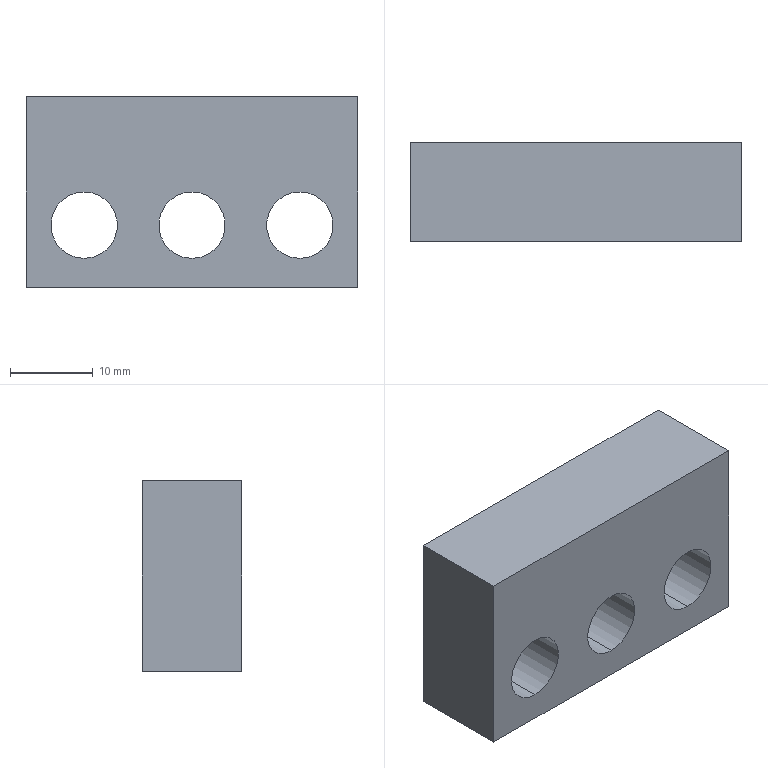Part | SolidWorks | features ICE 5, Extrusion 1 | 1 solid | 12 faces | box 40 x 12 x 23 mm | volume 9230 mm3 | cylinder 6 | plane 6 | commonest cylinder face diameters 8 x6
STEP:
#1=CARTESIAN_POINT('',(0.,6.,-4.));
#2=VERTEX_POINT('',#1);
#3=CARTESIAN_POINT('',(0.,6.,4.));
#4=VERTEX_POINT('',#3);
#5=CARTESIAN_POINT('',(0.,6.,0.));
#6=DIRECTION('',(0.,1.,0.));
#7=DIRECTION('',(0.,0.,-1.));
#8=AXIS2_PLACEMENT_3D('',#5,#6,#7);
#9=CIRCLE('',#8,4.);
#10=EDGE_CURVE('',#2,#4,#9,.T.);
#11=ORIENTED_EDGE('',*,*,#10,.T.);
#12=CARTESIAN_POINT('',(0.,-6.,4.));
#13=VERTEX_POINT('',#12);
#14=CARTESIAN_POINT('',(0.,6.001,4.));
#15=DIRECTION('',(0.,-1.,0.));
#16=VECTOR('',#15,1000.);
#17=LINE('',#14,#16);
#18=EDGE_CURVE('',#4,#13,#17,.T.);
#19=ORIENTED_EDGE('',*,*,#18,.T.);
#20=CARTESIAN_POINT('',(0.,-6.,-4.));
#21=VERTEX_POINT('',#20);
#22=CARTESIAN_POINT('',(0.,-6.,0.));
#23=DIRECTION('',(0.,-1.,0.));
#24=DIRECTION('',(0.,0.,-1.));
#25=AXIS2_PLACEMENT_3D('',#22,#23,#24);
#26=CIRCLE('',#25,4.);
#27=EDGE_CURVE('',#13,#21,#26,.T.);
#28=ORIENTED_EDGE('',*,*,#27,.T.);
#29=CARTESIAN_POINT('',(0.,6.001,-4.));
#30=DIRECTION('',(0.,-1.,0.));
#31=VECTOR('',#30,1000.);
#32=LINE('',#29,#31);
#33=EDGE_CURVE('',#2,#21,#32,.T.);
#34=ORIENTED_EDGE('',*,*,#33,.F.);
#35=EDGE_LOOP('',(#11,#19,#28,#34));
#36=FACE_OUTER_BOUND('',#35,.T.);
#37=CARTESIAN_POINT('',(0.,6.001,0.));
#38=DIRECTION('',(0.,-1.,0.));
#39=DIRECTION('',(0.,0.,-1.));
#40=AXIS2_PLACEMENT_3D('',#37,#38,#39);
#41=CYLINDRICAL_SURFACE('',#40,4.);
#42=ADVANCED_FACE('',(#36),#41,.F.);
#43=CARTESIAN_POINT('',(-13.,-6.,4.));
#44=VERTEX_POINT('',#43);
#45=CARTESIAN_POINT('',(-13.,-6.,-4.));
#46=VERTEX_POINT('',#45);
#47=CARTESIAN_POINT('',(-13.,-6.,0.));
#48=DIRECTION('',(0.,-1.,0.));
#49=DIRECTION('',(0.,0.,1.));
#50=AXIS2_PLACEMENT_3D('',#47,#48,#49);
#51=CIRCLE('',#50,4.);
#52=EDGE_CURVE('',#44,#46,#51,.T.);
#53=ORIENTED_EDGE('',*,*,#52,.T.);
#54=CARTESIAN_POINT('',(-13.,6.,-4.));
#55=VERTEX_POINT('',#54);
#56=CARTESIAN_POINT('',(-13.,-6.001,-4.));
#57=DIRECTION('',(0.,1.,0.));
#58=VECTOR('',#57,1000.);
#59=LINE('',#56,#58);
#60=EDGE_CURVE('',#46,#55,#59,.T.);
#61=ORIENTED_EDGE('',*,*,#60,.T.);
#62=CARTESIAN_POINT('',(-13.,6.,4.));
#63=VERTEX_POINT('',#62);
#64=CARTESIAN_POINT('',(-13.,6.,0.));
#65=DIRECTION('',(0.,1.,0.));
#66=DIRECTION('',(0.,0.,1.));
#67=AXIS2_PLACEMENT_3D('',#64,#65,#66);
#68=CIRCLE('',#67,4.);
#69=EDGE_CURVE('',#55,#63,#68,.T.);
#70=ORIENTED_EDGE('',*,*,#69,.T.);
#71=CARTESIAN_POINT('',(-13.,-6.001,4.));
#72=DIRECTION('',(0.,1.,0.));
#73=VECTOR('',#72,1000.);
#74=LINE('',#71,#73);
#75=EDGE_CURVE('',#44,#63,#74,.T.);
#76=ORIENTED_EDGE('',*,*,#75,.F.);
#77=EDGE_LOOP('',(#53,#61,#70,#76));
#78=FACE_OUTER_BOUND('',#77,.T.);
#79=CARTESIAN_POINT('',(-13.,-6.001,0.));
#80=DIRECTION('',(0.,1.,0.));
#81=DIRECTION('',(0.,0.,1.));
#82=AXIS2_PLACEMENT_3D('',#79,#80,#81);
#83=CYLINDRICAL_SURFACE('',#82,4.);
#84=ADVANCED_FACE('',(#78),#83,.F.);
#85=CARTESIAN_POINT('',(13.,-6.,4.));
#86=VERTEX_POINT('',#85);
#87=CARTESIAN_POINT('',(13.,-6.,-4.));
#88=VERTEX_POINT('',#87);
#89=CARTESIAN_POINT('',(13.,-6.,0.));
#90=DIRECTION('',(0.,-1.,0.));
#91=DIRECTION('',(0.,0.,1.));
#92=AXIS2_PLACEMENT_3D('',#89,#90,#91);
#93=CIRCLE('',#92,4.);
#94=EDGE_CURVE('',#86,#88,#93,.T.);
#95=ORIENTED_EDGE('',*,*,#94,.T.);
#96=CARTESIAN_POINT('',(13.,6.,-4.));
#97=VERTEX_POINT('',#96);
#98=CARTESIAN_POINT('',(13.,-6.001,-4.));
#99=DIRECTION('',(0.,1.,0.));
#100=VECTOR('',#99,1000.);
#101=LINE('',#98,#100);
#102=EDGE_CURVE('',#88,#97,#101,.T.);
#103=ORIENTED_EDGE('',*,*,#102,.T.);
#104=CARTESIAN_POINT('',(13.,6.,4.));
#105=VERTEX_POINT('',#104);
#106=CARTESIAN_POINT('',(13.,6.,0.));
#107=DIRECTION('',(0.,1.,0.));
#108=DIRECTION('',(0.,0.,1.));
#109=AXIS2_PLACEMENT_3D('',#106,#107,#108);
#110=CIRCLE('',#109,4.);
#111=EDGE_CURVE('',#97,#105,#110,.T.);
#112=ORIENTED_EDGE('',*,*,#111,.T.);
#113=CARTESIAN_POINT('',(13.,-6.001,4.));
#114=DIRECTION('',(0.,1.,0.));
#115=VECTOR('',#114,1000.);
#116=LINE('',#113,#115);
#117=EDGE_CURVE('',#86,#105,#116,.T.);
#118=ORIENTED_EDGE('',*,*,#117,.F.);
#119=EDGE_LOOP('',(#95,#103,#112,#118));
#120=FACE_OUTER_BOUND('',#119,.T.);
#121=CARTESIAN_POINT('',(13.,-6.001,0.));
#122=DIRECTION('',(0.,1.,0.));
#123=DIRECTION('',(0.,0.,1.));
#124=AXIS2_PLACEMENT_3D('',#121,#122,#123);
#125=CYLINDRICAL_SURFACE('',#124,4.);
#126=ADVANCED_FACE('',(#120),#125,.F.);
#127=CARTESIAN_POINT('',(20.,-6.,-7.5));
#128=VERTEX_POINT('',#127);
#129=CARTESIAN_POINT('',(20.,6.,-7.5));
#130=VERTEX_POINT('',#129);
#131=CARTESIAN_POINT('',(20.,-6.,-7.5));
#132=DIRECTION('',(0.,1.,0.));
#133=VECTOR('',#132,1000.);
#134=LINE('',#131,#133);
#135=EDGE_CURVE('',#128,#130,#134,.T.);
#136=ORIENTED_EDGE('',*,*,#135,.T.);
#137=CARTESIAN_POINT('',(20.,6.,15.5));
#138=VERTEX_POINT('',#137);
#139=CARTESIAN_POINT('',(20.,6.,7.5));
#140=DIRECTION('',(0.,0.,-1.));
#141=VECTOR('',#140,1000.);
#142=LINE('',#139,#141);
#143=EDGE_CURVE('',#138,#130,#142,.T.);
#144=ORIENTED_EDGE('',*,*,#143,.F.);
#145=CARTESIAN_POINT('',(20.,-6.,15.5));
#146=VERTEX_POINT('',#145);
#147=CARTESIAN_POINT('',(20.,-6.,15.5));
#148=DIRECTION('',(0.,1.,0.));
#149=VECTOR('',#148,1000.);
#150=LINE('',#147,#149);
#151=EDGE_CURVE('',#146,#138,#150,.T.);
#152=ORIENTED_EDGE('',*,*,#151,.F.);
#153=CARTESIAN_POINT('',(20.,-6.,7.5));
#154=DIRECTION('',(0.,0.,-1.));
#155=VECTOR('',#154,1000.);
#156=LINE('',#153,#155);
#157=EDGE_CURVE('',#146,#128,#156,.T.);
#158=ORIENTED_EDGE('',*,*,#157,.T.);
#159=EDGE_LOOP('',(#136,#144,#152,#158));
#160=FACE_OUTER_BOUND('',#159,.T.);
#161=CARTESIAN_POINT('',(20.,-6.,7.5));
#162=DIRECTION('',(-1.,0.,0.));
#163=DIRECTION('',(0.,0.,1.));
#164=AXIS2_PLACEMENT_3D('',#161,#162,#163);
#165=PLANE('',#164);
#166=ADVANCED_FACE('',(#160),#165,.F.);
#167=ORIENTED_EDGE('',*,*,#10,.F.);
#168=CARTESIAN_POINT('',(0.,6.,0.));
#169=DIRECTION('',(0.,1.,0.));
#170=DIRECTION('',(0.,0.,-1.));
#171=AXIS2_PLACEMENT_3D('',#168,#169,#170);
#172=CIRCLE('',#171,4.);
#173=EDGE_CURVE('',#4,#2,#172,.T.);
#174=ORIENTED_EDGE('',*,*,#173,.F.);
#175=EDGE_LOOP('',(#167,#174));
#176=FACE_BOUND('',#175,.T.);
#177=CARTESIAN_POINT('',(-13.,6.,0.));
#178=DIRECTION('',(0.,1.,0.));
#179=DIRECTION('',(0.,0.,1.));
#180=AXIS2_PLACEMENT_3D('',#177,#178,#179);
#181=CIRCLE('',#180,4.);
#182=EDGE_CURVE('',#63,#55,#181,.T.);
#183=ORIENTED_EDGE('',*,*,#182,.F.);
#184=ORIENTED_EDGE('',*,*,#69,.F.);
#185=EDGE_LOOP('',(#183,#184));
#186=FACE_BOUND('',#185,.T.);
#187=CARTESIAN_POINT('',(13.,6.,0.));
#188=DIRECTION('',(0.,1.,0.));
#189=DIRECTION('',(0.,0.,1.));
#190=AXIS2_PLACEMENT_3D('',#187,#188,#189);
#191=CIRCLE('',#190,4.);
#192=EDGE_CURVE('',#105,#97,#191,.T.);
#193=ORIENTED_EDGE('',*,*,#192,.F.);
#194=ORIENTED_EDGE('',*,*,#111,.F.);
#195=EDGE_LOOP('',(#193,#194));
#196=FACE_BOUND('',#195,.T.);
#197=CARTESIAN_POINT('',(-20.,6.,-7.5));
#198=VERTEX_POINT('',#197);
#199=CARTESIAN_POINT('',(-20.,6.,-7.5));
#200=DIRECTION('',(-1.,0.,0.));
#201=VECTOR('',#200,1000.);
#202=LINE('',#199,#201);
#203=EDGE_CURVE('',#130,#198,#202,.T.);
#204=ORIENTED_EDGE('',*,*,#203,.T.);
#205=CARTESIAN_POINT('',(-20.,6.,15.5));
#206=VERTEX_POINT('',#205);
#207=CARTESIAN_POINT('',(-20.,6.,7.5));
#208=DIRECTION('',(0.,0.,-1.));
#209=VECTOR('',#208,1000.);
#210=LINE('',#207,#209);
#211=EDGE_CURVE('',#206,#198,#210,.T.);
#212=ORIENTED_EDGE('',*,*,#211,.F.);
#213=CARTESIAN_POINT('',(-20.,6.,15.5));
#214=DIRECTION('',(-1.,0.,0.));
#215=VECTOR('',#214,1000.);
#216=LINE('',#213,#215);
#217=EDGE_CURVE('',#138,#206,#216,.T.);
#218=ORIENTED_EDGE('',*,*,#217,.F.);
#219=ORIENTED_EDGE('',*,*,#143,.T.);
#220=EDGE_LOOP('',(#204,#212,#218,#219));
#221=FACE_OUTER_BOUND('',#220,.T.);
#222=CARTESIAN_POINT('',(-20.,6.,7.5));
#223=DIRECTION('',(0.,-1.,0.));
#224=DIRECTION('',(0.,0.,-1.));
#225=AXIS2_PLACEMENT_3D('',#222,#223,#224);
#226=PLANE('',#225);
#227=ADVANCED_FACE('',(#176,#186,#196,#221),#226,.F.);
#228=CARTESIAN_POINT('',(-20.,-6.,-7.5));
#229=VERTEX_POINT('',#228);
#230=CARTESIAN_POINT('',(-20.,-6.,-7.5));
#231=DIRECTION('',(0.,-1.,0.));
#232=VECTOR('',#231,1000.);
#233=LINE('',#230,#232);
#234=EDGE_CURVE('',#198,#229,#233,.T.);
#235=ORIENTED_EDGE('',*,*,#234,.T.);
#236=CARTESIAN_POINT('',(-20.,-6.,15.5));
#237=VERTEX_POINT('',#236);
#238=CARTESIAN_POINT('',(-20.,-6.,7.5));
#239=DIRECTION('',(0.,0.,-1.));
#240=VECTOR('',#239,1000.);
#241=LINE('',#238,#240);
#242=EDGE_CURVE('',#237,#229,#241,.T.);
#243=ORIENTED_EDGE('',*,*,#242,.F.);
#244=CARTESIAN_POINT('',(-20.,-6.,15.5));
#245=DIRECTION('',(0.,-1.,0.));
#246=VECTOR('',#245,1000.);
#247=LINE('',#244,#246);
#248=EDGE_CURVE('',#206,#237,#247,.T.);
#249=ORIENTED_EDGE('',*,*,#248,.F.);
#250=ORIENTED_EDGE('',*,*,#211,.T.);
#251=EDGE_LOOP('',(#235,#243,#249,#250));
#252=FACE_OUTER_BOUND('',#251,.T.);
#253=CARTESIAN_POINT('',(-20.,-6.,7.5));
#254=DIRECTION('',(1.,0.,0.));
#255=DIRECTION('',(0.,0.,-1.));
#256=AXIS2_PLACEMENT_3D('',#253,#254,#255);
#257=PLANE('',#256);
#258=ADVANCED_FACE('',(#252),#257,.F.);
#259=CARTESIAN_POINT('',(0.,-6.,0.));
#260=DIRECTION('',(0.,-1.,0.));
#261=DIRECTION('',(0.,0.,-1.));
#262=AXIS2_PLACEMENT_3D('',#259,#260,#261);
#263=CIRCLE('',#262,4.);
#264=EDGE_CURVE('',#21,#13,#263,.T.);
#265=ORIENTED_EDGE('',*,*,#264,.F.);
#266=ORIENTED_EDGE('',*,*,#27,.F.);
#267=EDGE_LOOP('',(#265,#266));
#268=FACE_BOUND('',#267,.T.);
#269=ORIENTED_EDGE('',*,*,#52,.F.);
#270=CARTESIAN_POINT('',(-13.,-6.,0.));
#271=DIRECTION('',(0.,-1.,0.));
#272=DIRECTION('',(0.,0.,1.));
#273=AXIS2_PLACEMENT_3D('',#270,#271,#272);
#274=CIRCLE('',#273,4.);
#275=EDGE_CURVE('',#46,#44,#274,.T.);
#276=ORIENTED_EDGE('',*,*,#275,.F.);
#277=EDGE_LOOP('',(#269,#276));
#278=FACE_BOUND('',#277,.T.);
#279=ORIENTED_EDGE('',*,*,#94,.F.);
#280=CARTESIAN_POINT('',(13.,-6.,0.));
#281=DIRECTION('',(0.,-1.,0.));
#282=DIRECTION('',(0.,0.,1.));
#283=AXIS2_PLACEMENT_3D('',#280,#281,#282);
#284=CIRCLE('',#283,4.);
#285=EDGE_CURVE('',#88,#86,#284,.T.);
#286=ORIENTED_EDGE('',*,*,#285,.F.);
#287=EDGE_LOOP('',(#279,#286));
#288=FACE_BOUND('',#287,.T.);
#289=CARTESIAN_POINT('',(-20.,-6.,-7.5));
#290=DIRECTION('',(1.,0.,0.));
#291=VECTOR('',#290,1000.);
#292=LINE('',#289,#291);
#293=EDGE_CURVE('',#229,#128,#292,.T.);
#294=ORIENTED_EDGE('',*,*,#293,.T.);
#295=ORIENTED_EDGE('',*,*,#157,.F.);
#296=CARTESIAN_POINT('',(-20.,-6.,15.5));
#297=DIRECTION('',(1.,0.,0.));
#298=VECTOR('',#297,1000.);
#299=LINE('',#296,#298);
#300=EDGE_CURVE('',#237,#146,#299,.T.);
#301=ORIENTED_EDGE('',*,*,#300,.F.);
#302=ORIENTED_EDGE('',*,*,#242,.T.);
#303=EDGE_LOOP('',(#294,#295,#301,#302));
#304=FACE_OUTER_BOUND('',#303,.T.);
#305=CARTESIAN_POINT('',(-20.,-6.,7.5));
#306=DIRECTION('',(0.,1.,0.));
#307=DIRECTION('',(0.,0.,1.));
#308=AXIS2_PLACEMENT_3D('',#305,#306,#307);
#309=PLANE('',#308);
#310=ADVANCED_FACE('',(#268,#278,#288,#304),#309,.F.);
#311=ORIENTED_EDGE('',*,*,#135,.F.);
#312=ORIENTED_EDGE('',*,*,#293,.F.);
#313=ORIENTED_EDGE('',*,*,#234,.F.);
#314=ORIENTED_EDGE('',*,*,#203,.F.);
#315=EDGE_LOOP('',(#311,#312,#313,#314));
#316=FACE_OUTER_BOUND('',#315,.T.);
#317=CARTESIAN_POINT('',(0.,0.,-7.5));
#318=DIRECTION('',(0.,0.,-1.));
#319=DIRECTION('',(-1.,0.,0.));
#320=AXIS2_PLACEMENT_3D('',#317,#318,#319);
#321=PLANE('',#320);
#322=ADVANCED_FACE('',(#316),#321,.T.);
#323=ORIENTED_EDGE('',*,*,#102,.F.);
#324=ORIENTED_EDGE('',*,*,#285,.T.);
#325=ORIENTED_EDGE('',*,*,#117,.T.);
#326=ORIENTED_EDGE('',*,*,#192,.T.);
#327=EDGE_LOOP('',(#323,#324,#325,#326));
#328=FACE_OUTER_BOUND('',#327,.T.);
#329=CARTESIAN_POINT('',(13.,-6.001,0.));
#330=DIRECTION('',(0.,1.,0.));
#331=DIRECTION('',(0.,0.,1.));
#332=AXIS2_PLACEMENT_3D('',#329,#330,#331);
#333=CYLINDRICAL_SURFACE('',#332,4.);
#334=ADVANCED_FACE('',(#328),#333,.F.);
#335=ORIENTED_EDGE('',*,*,#60,.F.);
#336=ORIENTED_EDGE('',*,*,#275,.T.);
#337=ORIENTED_EDGE('',*,*,#75,.T.);
#338=ORIENTED_EDGE('',*,*,#182,.T.);
#339=EDGE_LOOP('',(#335,#336,#337,#338));
#340=FACE_OUTER_BOUND('',#339,.T.);
#341=CARTESIAN_POINT('',(-13.,-6.001,0.));
#342=DIRECTION('',(0.,1.,0.));
#343=DIRECTION('',(0.,0.,1.));
#344=AXIS2_PLACEMENT_3D('',#341,#342,#343);
#345=CYLINDRICAL_SURFACE('',#344,4.);
#346=ADVANCED_FACE('',(#340),#345,.F.);
#347=ORIENTED_EDGE('',*,*,#18,.F.);
#348=ORIENTED_EDGE('',*,*,#173,.T.);
#349=ORIENTED_EDGE('',*,*,#33,.T.);
#350=ORIENTED_EDGE('',*,*,#264,.T.);
#351=EDGE_LOOP('',(#347,#348,#349,#350));
#352=FACE_OUTER_BOUND('',#351,.T.);
#353=CARTESIAN_POINT('',(0.,6.001,0.));
#354=DIRECTION('',(0.,-1.,0.));
#355=DIRECTION('',(0.,0.,-1.));
#356=AXIS2_PLACEMENT_3D('',#353,#354,#355);
#357=CYLINDRICAL_SURFACE('',#356,4.);
#358=ADVANCED_FACE('',(#352),#357,.F.);
#359=ORIENTED_EDGE('',*,*,#248,.T.);
#360=ORIENTED_EDGE('',*,*,#300,.T.);
#361=ORIENTED_EDGE('',*,*,#151,.T.);
#362=ORIENTED_EDGE('',*,*,#217,.T.);
#363=EDGE_LOOP('',(#359,#360,#361,#362));
#364=FACE_OUTER_BOUND('',#363,.T.);
#365=CARTESIAN_POINT('',(0.,0.,15.5));
#366=DIRECTION('',(0.,0.,-1.));
#367=DIRECTION('',(-1.,0.,0.));
#368=AXIS2_PLACEMENT_3D('',#365,#366,#367);
#369=PLANE('',#368);
#370=ADVANCED_FACE('',(#364),#369,.F.);
#371=CLOSED_SHELL('',(#42,#84,#126,#166,#227,#258,#310,#322,#334,#346,#358,#370));
#372=MANIFOLD_SOLID_BREP('',#371);
#373=CARTESIAN_POINT('',(0.,0.,0.));
#374=DIRECTION('',(0.,0.,1.));
#375=DIRECTION('',(1.,0.,0.));
#376=AXIS2_PLACEMENT_3D('',#373,#374,#375);
#377=(LENGTH_UNIT()NAMED_UNIT(*)SI_UNIT(.MILLI.,.METRE.));
#378=UNCERTAINTY_MEASURE_WITH_UNIT(LENGTH_MEASURE(0.00001),#377,'','');
#379=(NAMED_UNIT(*)PLANE_ANGLE_UNIT()SI_UNIT($,.RADIAN.));
#380=(NAMED_UNIT(*)SI_UNIT($,.STERADIAN.)SOLID_ANGLE_UNIT());
#381=(GEOMETRIC_REPRESENTATION_CONTEXT(3)GLOBAL_UNCERTAINTY_ASSIGNED_CONTEXT((#378))GLOBAL_UNIT_ASSIGNED_CONTEXT((#377,#379,#380))REPRESENTATION_CONTEXT('',''));
#382=ADVANCED_BREP_SHAPE_REPRESENTATION('',(#372,#376),#381);